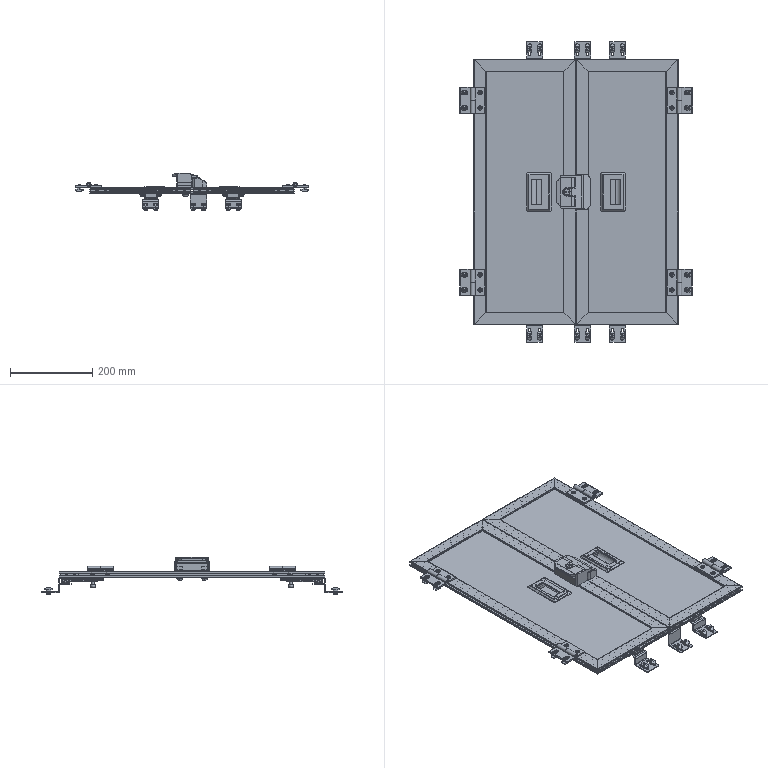Part | NX | features BREP 38 | 204 solids | 4860 faces | volume 2441373 mm3 | plane 2683 | cylinder 1481 | cone 560 | torus 102 | sphere 34 | commonest cylinder face diameters 5 x412 6 x114 4 x101 8 x96 1 x87 2 x73